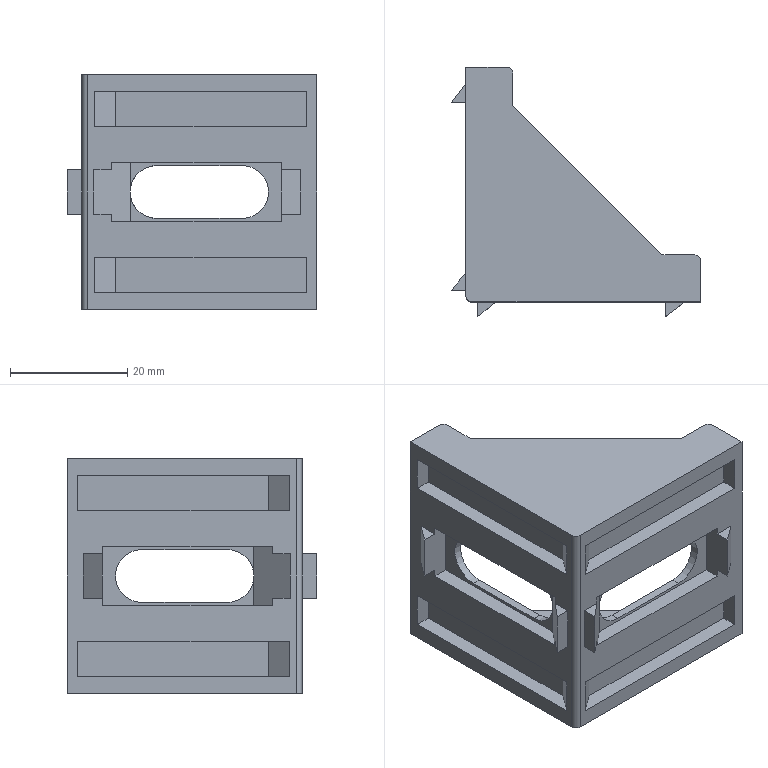Part | SolidWorks | features ICE 7, Extrusion 1, Fillet 1, LPattern 1, MirrorPattern 1 | 1 solid | 72 faces | box 42.5 x 42.5 x 40 mm | volume 12926 mm3 | plane 62 | cylinder 10 | commonest cylinder face diameters 2 x5 9 x5